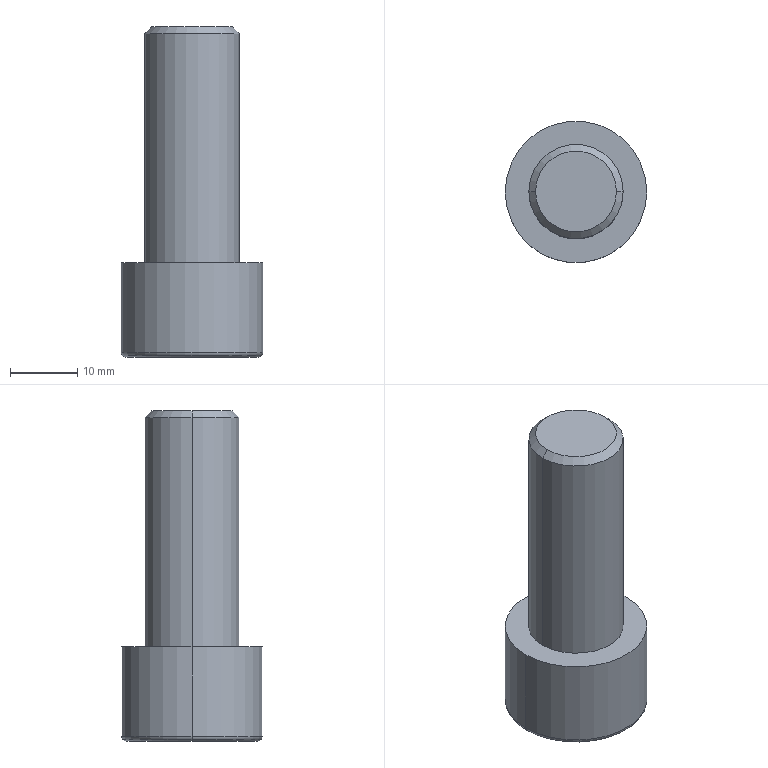Part | Creo | 1 solid | 20 faces | box 21 x 21 x 49 mm | volume 9057 mm3 | plane 10 | cylinder 4 | torus 4 | cone 2 | commonest cylinder face diameters 14 x2 21 x2
STEP:
#1=CARTESIAN_POINT('',(-272.,347.,-256.5));
#2=VERTEX_POINT('',#1);
#3=CARTESIAN_POINT('',(-258.,347.,-256.5));
#4=VERTEX_POINT('',#3);
#5=CARTESIAN_POINT('',(-265.,347.,-256.5));
#6=DIRECTION('',(0.,0.,1.));
#7=DIRECTION('',(-1.,0.,0.));
#8=AXIS2_PLACEMENT_3D('',#5,#6,#7);
#9=CIRCLE('',#8,7.);
#10=EDGE_CURVE('',#2,#4,#9,.T.);
#11=ORIENTED_EDGE('',*,*,#10,.T.);
#12=CARTESIAN_POINT('',(-258.,347.,-290.5));
#13=VERTEX_POINT('',#12);
#14=CARTESIAN_POINT('',(-258.,347.,-290.5));
#15=DIRECTION('',(0.,0.,1.));
#16=VECTOR('',#15,34.);
#17=LINE('',#14,#16);
#18=EDGE_CURVE('',#13,#4,#17,.T.);
#19=ORIENTED_EDGE('',*,*,#18,.F.);
#20=CARTESIAN_POINT('',(-272.,347.,-290.5));
#21=VERTEX_POINT('',#20);
#22=CARTESIAN_POINT('',(-265.,347.,-290.5));
#23=DIRECTION('',(0.,0.,-1.));
#24=DIRECTION('',(1.,0.,0.));
#25=AXIS2_PLACEMENT_3D('',#22,#23,#24);
#26=CIRCLE('',#25,7.);
#27=EDGE_CURVE('',#13,#21,#26,.T.);
#28=ORIENTED_EDGE('',*,*,#27,.T.);
#29=CARTESIAN_POINT('',(-272.,347.,-290.5));
#30=DIRECTION('',(0.,0.,1.));
#31=VECTOR('',#30,34.);
#32=LINE('',#29,#31);
#33=EDGE_CURVE('',#21,#2,#32,.T.);
#34=ORIENTED_EDGE('',*,*,#33,.T.);
#35=EDGE_LOOP('',(#11,#19,#28,#34));
#36=FACE_OUTER_BOUND('',#35,.F.);
#37=CARTESIAN_POINT('',(-265.,347.,-290.5));
#38=DIRECTION('',(0.,0.,1.));
#39=DIRECTION('',(-1.,0.,0.));
#40=AXIS2_PLACEMENT_3D('',#37,#38,#39);
#41=CYLINDRICAL_SURFACE('',#40,7.);
#42=ADVANCED_FACE('',(#36),#41,.T.);
#43=CARTESIAN_POINT('',(-271.,347.,-255.5));
#44=VERTEX_POINT('',#43);
#45=CARTESIAN_POINT('',(-259.,347.,-255.5));
#46=VERTEX_POINT('',#45);
#47=CARTESIAN_POINT('',(-265.,347.,-255.5));
#48=DIRECTION('',(0.,0.,1.));
#49=DIRECTION('',(-1.,0.,0.));
#50=AXIS2_PLACEMENT_3D('',#47,#48,#49);
#51=CIRCLE('',#50,6.);
#52=EDGE_CURVE('',#44,#46,#51,.T.);
#53=ORIENTED_EDGE('',*,*,#52,.T.);
#54=CARTESIAN_POINT('',(-259.,347.,-255.5));
#55=DIRECTION('',(0.7071,0.,-0.7071));
#56=VECTOR('',#55,1.414);
#57=LINE('',#54,#56);
#58=EDGE_CURVE('',#46,#4,#57,.T.);
#59=ORIENTED_EDGE('',*,*,#58,.T.);
#60=ORIENTED_EDGE('',*,*,#10,.F.);
#61=CARTESIAN_POINT('',(-271.,347.,-255.5));
#62=DIRECTION('',(-0.7071,0.,-0.7071));
#63=VECTOR('',#62,1.414);
#64=LINE('',#61,#63);
#65=EDGE_CURVE('',#44,#2,#64,.T.);
#66=ORIENTED_EDGE('',*,*,#65,.F.);
#67=EDGE_LOOP('',(#53,#59,#60,#66));
#68=FACE_OUTER_BOUND('',#67,.F.);
#69=CARTESIAN_POINT('',(-265.,347.,-256.));
#70=DIRECTION('',(0.,0.,-1.));
#71=DIRECTION('',(1.,0.,0.));
#72=AXIS2_PLACEMENT_3D('',#69,#70,#71);
#73=CONICAL_SURFACE('',#72,6.5,45.);
#74=ADVANCED_FACE('',(#68),#73,.T.);
#75=CARTESIAN_POINT('',(-265.,347.,-255.5));
#76=DIRECTION('',(0.,0.,1.));
#77=DIRECTION('',(1.,0.,0.));
#78=AXIS2_PLACEMENT_3D('',#75,#76,#77);
#79=CIRCLE('',#78,6.);
#80=EDGE_CURVE('',#46,#44,#79,.T.);
#81=ORIENTED_EDGE('',*,*,#80,.F.);
#82=ORIENTED_EDGE('',*,*,#52,.F.);
#83=EDGE_LOOP('',(#81,#82));
#84=FACE_OUTER_BOUND('',#83,.F.);
#85=CARTESIAN_POINT('',(-265.,347.,-255.5));
#86=DIRECTION('',(0.,0.,-1.));
#87=DIRECTION('',(1.,0.,0.));
#88=AXIS2_PLACEMENT_3D('',#85,#86,#87);
#89=PLANE('',#88);
#90=ADVANCED_FACE('',(#84),#89,.F.);
#91=ORIENTED_EDGE('',*,*,#80,.T.);
#92=ORIENTED_EDGE('',*,*,#65,.T.);
#93=CARTESIAN_POINT('',(-265.,347.,-256.5));
#94=DIRECTION('',(0.,0.,1.));
#95=DIRECTION('',(1.,0.,0.));
#96=AXIS2_PLACEMENT_3D('',#93,#94,#95);
#97=CIRCLE('',#96,7.);
#98=EDGE_CURVE('',#4,#2,#97,.T.);
#99=ORIENTED_EDGE('',*,*,#98,.F.);
#100=ORIENTED_EDGE('',*,*,#58,.F.);
#101=EDGE_LOOP('',(#91,#92,#99,#100));
#102=FACE_OUTER_BOUND('',#101,.F.);
#103=CARTESIAN_POINT('',(-265.,347.,-256.));
#104=DIRECTION('',(0.,0.,-1.));
#105=DIRECTION('',(1.,0.,0.));
#106=AXIS2_PLACEMENT_3D('',#103,#104,#105);
#107=CONICAL_SURFACE('',#106,6.5,45.);
#108=ADVANCED_FACE('',(#102),#107,.T.);
#109=ORIENTED_EDGE('',*,*,#98,.T.);
#110=ORIENTED_EDGE('',*,*,#33,.F.);
#111=CARTESIAN_POINT('',(-265.,347.,-290.5));
#112=DIRECTION('',(0.,0.,-1.));
#113=DIRECTION('',(-1.,0.,0.));
#114=AXIS2_PLACEMENT_3D('',#111,#112,#113);
#115=CIRCLE('',#114,7.);
#116=EDGE_CURVE('',#21,#13,#115,.T.);
#117=ORIENTED_EDGE('',*,*,#116,.T.);
#118=ORIENTED_EDGE('',*,*,#18,.T.);
#119=EDGE_LOOP('',(#109,#110,#117,#118));
#120=FACE_OUTER_BOUND('',#119,.F.);
#121=CARTESIAN_POINT('',(-265.,347.,-290.5));
#122=DIRECTION('',(0.,0.,1.));
#123=DIRECTION('',(-1.,0.,0.));
#124=AXIS2_PLACEMENT_3D('',#121,#122,#123);
#125=CYLINDRICAL_SURFACE('',#124,7.);
#126=ADVANCED_FACE('',(#120),#125,.T.);
#127=CARTESIAN_POINT('',(-254.5,347.,-290.5));
#128=VERTEX_POINT('',#127);
#129=CARTESIAN_POINT('',(-275.5,347.,-290.5));
#130=VERTEX_POINT('',#129);
#131=CARTESIAN_POINT('',(-265.,347.,-290.5));
#132=DIRECTION('',(0.,0.,1.));
#133=DIRECTION('',(1.,0.,0.));
#134=AXIS2_PLACEMENT_3D('',#131,#132,#133);
#135=CIRCLE('',#134,10.5);
#136=EDGE_CURVE('',#128,#130,#135,.T.);
#137=ORIENTED_EDGE('',*,*,#136,.F.);
#138=CARTESIAN_POINT('',(-265.,347.,-290.5));
#139=DIRECTION('',(0.,0.,1.));
#140=DIRECTION('',(-1.,0.,0.));
#141=AXIS2_PLACEMENT_3D('',#138,#139,#140);
#142=CIRCLE('',#141,10.5);
#143=EDGE_CURVE('',#130,#128,#142,.T.);
#144=ORIENTED_EDGE('',*,*,#143,.F.);
#145=EDGE_LOOP('',(#137,#144));
#146=FACE_OUTER_BOUND('',#145,.F.);
#147=ORIENTED_EDGE('',*,*,#27,.F.);
#148=ORIENTED_EDGE('',*,*,#116,.F.);
#149=EDGE_LOOP('',(#147,#148));
#150=FACE_BOUND('',#149,.F.);
#151=CARTESIAN_POINT('',(-265.,347.,-290.5));
#152=DIRECTION('',(0.,0.,1.));
#153=DIRECTION('',(-1.,0.,0.));
#154=AXIS2_PLACEMENT_3D('',#151,#152,#153);
#155=PLANE('',#154);
#156=ADVANCED_FACE('',(#146,#150),#155,.T.);
#157=CARTESIAN_POINT('',(-275.5,347.,-303.8));
#158=VERTEX_POINT('',#157);
#159=CARTESIAN_POINT('',(-254.5,347.,-303.8));
#160=VERTEX_POINT('',#159);
#161=CARTESIAN_POINT('',(-265.,347.,-303.8));
#162=DIRECTION('',(0.,0.,-1.));
#163=DIRECTION('',(-1.,0.,0.));
#164=AXIS2_PLACEMENT_3D('',#161,#162,#163);
#165=CIRCLE('',#164,10.5);
#166=EDGE_CURVE('',#158,#160,#165,.T.);
#167=ORIENTED_EDGE('',*,*,#166,.T.);
#168=CARTESIAN_POINT('',(-254.5,347.,-290.5));
#169=DIRECTION('',(0.,0.,-1.));
#170=VECTOR('',#169,13.3);
#171=LINE('',#168,#170);
#172=EDGE_CURVE('',#128,#160,#171,.T.);
#173=ORIENTED_EDGE('',*,*,#172,.F.);
#174=ORIENTED_EDGE('',*,*,#136,.T.);
#175=CARTESIAN_POINT('',(-275.5,347.,-290.5));
#176=DIRECTION('',(0.,0.,-1.));
#177=VECTOR('',#176,13.3);
#178=LINE('',#175,#177);
#179=EDGE_CURVE('',#130,#158,#178,.T.);
#180=ORIENTED_EDGE('',*,*,#179,.T.);
#181=EDGE_LOOP('',(#167,#173,#174,#180));
#182=FACE_OUTER_BOUND('',#181,.F.);
#183=CARTESIAN_POINT('',(-265.,347.,-290.5));
#184=DIRECTION('',(0.,0.,-1.));
#185=DIRECTION('',(1.,0.,0.));
#186=AXIS2_PLACEMENT_3D('',#183,#184,#185);
#187=CYLINDRICAL_SURFACE('',#186,10.5);
#188=ADVANCED_FACE('',(#182),#187,.T.);
#189=ORIENTED_EDGE('',*,*,#166,.F.);
#190=CARTESIAN_POINT('',(-275.295,347.,-304.295));
#191=VERTEX_POINT('',#190);
#192=CARTESIAN_POINT('',(-274.8,347.,-303.8));
#193=DIRECTION('',(0.,-1.,0.));
#194=DIRECTION('',(-1.,0.,0.));
#195=AXIS2_PLACEMENT_3D('',#192,#193,#194);
#196=CIRCLE('',#195,0.7);
#197=EDGE_CURVE('',#158,#191,#196,.T.);
#198=ORIENTED_EDGE('',*,*,#197,.T.);
#199=CARTESIAN_POINT('',(-254.705,347.,-304.295));
#200=VERTEX_POINT('',#199);
#201=CARTESIAN_POINT('',(-265.,347.,-304.295));
#202=DIRECTION('',(0.,0.,-1.));
#203=DIRECTION('',(-1.,0.,0.));
#204=AXIS2_PLACEMENT_3D('',#201,#202,#203);
#205=CIRCLE('',#204,10.295);
#206=EDGE_CURVE('',#191,#200,#205,.T.);
#207=ORIENTED_EDGE('',*,*,#206,.T.);
#208=CARTESIAN_POINT('',(-255.2,347.,-303.8));
#209=DIRECTION('',(0.,1.,0.));
#210=DIRECTION('',(1.,0.,0.));
#211=AXIS2_PLACEMENT_3D('',#208,#209,#210);
#212=CIRCLE('',#211,0.7);
#213=EDGE_CURVE('',#160,#200,#212,.T.);
#214=ORIENTED_EDGE('',*,*,#213,.F.);
#215=EDGE_LOOP('',(#189,#198,#207,#214));
#216=FACE_OUTER_BOUND('',#215,.F.);
#217=CARTESIAN_POINT('',(-265.,347.,-303.8));
#218=DIRECTION('',(0.,0.,-1.));
#219=DIRECTION('',(1.,0.,0.));
#220=AXIS2_PLACEMENT_3D('',#217,#218,#219);
#221=TOROIDAL_SURFACE('',#220,9.8,0.7);
#222=ADVANCED_FACE('',(#216),#221,.T.);
#223=CARTESIAN_POINT('',(-265.,347.,-303.8));
#224=DIRECTION('',(0.,0.,-1.));
#225=DIRECTION('',(1.,0.,0.));
#226=AXIS2_PLACEMENT_3D('',#223,#224,#225);
#227=CIRCLE('',#226,10.5);
#228=EDGE_CURVE('',#160,#158,#227,.T.);
#229=ORIENTED_EDGE('',*,*,#228,.F.);
#230=ORIENTED_EDGE('',*,*,#213,.T.);
#231=CARTESIAN_POINT('',(-265.,347.,-304.295));
#232=DIRECTION('',(0.,0.,-1.));
#233=DIRECTION('',(1.,0.,0.));
#234=AXIS2_PLACEMENT_3D('',#231,#232,#233);
#235=CIRCLE('',#234,10.295);
#236=EDGE_CURVE('',#200,#191,#235,.T.);
#237=ORIENTED_EDGE('',*,*,#236,.T.);
#238=ORIENTED_EDGE('',*,*,#197,.F.);
#239=EDGE_LOOP('',(#229,#230,#237,#238));
#240=FACE_OUTER_BOUND('',#239,.F.);
#241=CARTESIAN_POINT('',(-265.,347.,-303.8));
#242=DIRECTION('',(0.,0.,-1.));
#243=DIRECTION('',(1.,0.,0.));
#244=AXIS2_PLACEMENT_3D('',#241,#242,#243);
#245=TOROIDAL_SURFACE('',#244,9.8,0.7);
#246=ADVANCED_FACE('',(#240),#245,.T.);
#247=ORIENTED_EDGE('',*,*,#228,.T.);
#248=ORIENTED_EDGE('',*,*,#179,.F.);
#249=ORIENTED_EDGE('',*,*,#143,.T.);
#250=ORIENTED_EDGE('',*,*,#172,.T.);
#251=EDGE_LOOP('',(#247,#248,#249,#250));
#252=FACE_OUTER_BOUND('',#251,.F.);
#253=CARTESIAN_POINT('',(-265.,347.,-290.5));
#254=DIRECTION('',(0.,0.,-1.));
#255=DIRECTION('',(1.,0.,0.));
#256=AXIS2_PLACEMENT_3D('',#253,#254,#255);
#257=CYLINDRICAL_SURFACE('',#256,10.5);
#258=ADVANCED_FACE('',(#252),#257,.T.);
#259=CARTESIAN_POINT('',(-255.2,347.,-304.5));
#260=VERTEX_POINT('',#259);
#261=CARTESIAN_POINT('',(-274.8,347.,-304.5));
#262=VERTEX_POINT('',#261);
#263=CARTESIAN_POINT('',(-265.,347.,-304.5));
#264=DIRECTION('',(0.,0.,-1.));
#265=DIRECTION('',(1.,0.,0.));
#266=AXIS2_PLACEMENT_3D('',#263,#264,#265);
#267=CIRCLE('',#266,9.8);
#268=EDGE_CURVE('',#260,#262,#267,.T.);
#269=ORIENTED_EDGE('',*,*,#268,.T.);
#270=CARTESIAN_POINT('',(-274.8,347.,-303.8));
#271=DIRECTION('',(0.,-1.,0.));
#272=DIRECTION('',(-0.7071,0.,-0.7071));
#273=AXIS2_PLACEMENT_3D('',#270,#271,#272);
#274=CIRCLE('',#273,0.7);
#275=EDGE_CURVE('',#191,#262,#274,.T.);
#276=ORIENTED_EDGE('',*,*,#275,.F.);
#277=ORIENTED_EDGE('',*,*,#236,.F.);
#278=CARTESIAN_POINT('',(-255.2,347.,-303.8));
#279=DIRECTION('',(0.,1.,0.));
#280=DIRECTION('',(0.7071,0.,-0.7071));
#281=AXIS2_PLACEMENT_3D('',#278,#279,#280);
#282=CIRCLE('',#281,0.7);
#283=EDGE_CURVE('',#200,#260,#282,.T.);
#284=ORIENTED_EDGE('',*,*,#283,.T.);
#285=EDGE_LOOP('',(#269,#276,#277,#284));
#286=FACE_OUTER_BOUND('',#285,.F.);
#287=CARTESIAN_POINT('',(-265.,347.,-303.8));
#288=DIRECTION('',(0.,0.,-1.));
#289=DIRECTION('',(1.,0.,0.));
#290=AXIS2_PLACEMENT_3D('',#287,#288,#289);
#291=TOROIDAL_SURFACE('',#290,9.8,0.7);
#292=ADVANCED_FACE('',(#286),#291,.T.);
#293=ORIENTED_EDGE('',*,*,#268,.F.);
#294=CARTESIAN_POINT('',(-265.,347.,-304.5));
#295=DIRECTION('',(0.,0.,-1.));
#296=DIRECTION('',(-1.,0.,0.));
#297=AXIS2_PLACEMENT_3D('',#294,#295,#296);
#298=CIRCLE('',#297,9.8);
#299=EDGE_CURVE('',#262,#260,#298,.T.);
#300=ORIENTED_EDGE('',*,*,#299,.F.);
#301=EDGE_LOOP('',(#293,#300));
#302=FACE_OUTER_BOUND('',#301,.F.);
#303=CARTESIAN_POINT('',(-261.536,353.,-304.5));
#304=VERTEX_POINT('',#303);
#305=CARTESIAN_POINT('',(-268.464,353.,-304.5));
#306=VERTEX_POINT('',#305);
#307=CARTESIAN_POINT('',(-261.536,353.,-304.5));
#308=DIRECTION('',(-1.,0.,0.));
#309=VECTOR('',#308,6.928);
#310=LINE('',#307,#309);
#311=EDGE_CURVE('',#304,#306,#310,.T.);
#312=ORIENTED_EDGE('',*,*,#311,.F.);
#313=CARTESIAN_POINT('',(-258.072,347.,-304.5));
#314=VERTEX_POINT('',#313);
#315=CARTESIAN_POINT('',(-258.072,347.,-304.5));
#316=DIRECTION('',(-0.5,0.866,0.));
#317=VECTOR('',#316,6.928);
#318=LINE('',#315,#317);
#319=EDGE_CURVE('',#314,#304,#318,.T.);
#320=ORIENTED_EDGE('',*,*,#319,.F.);
#321=CARTESIAN_POINT('',(-261.536,341.,-304.5));
#322=VERTEX_POINT('',#321);
#323=CARTESIAN_POINT('',(-261.536,341.,-304.5));
#324=DIRECTION('',(0.5,0.866,0.));
#325=VECTOR('',#324,6.928);
#326=LINE('',#323,#325);
#327=EDGE_CURVE('',#322,#314,#326,.T.);
#328=ORIENTED_EDGE('',*,*,#327,.F.);
#329=CARTESIAN_POINT('',(-268.464,341.,-304.5));
#330=VERTEX_POINT('',#329);
#331=CARTESIAN_POINT('',(-268.464,341.,-304.5));
#332=DIRECTION('',(1.,0.,0.));
#333=VECTOR('',#332,6.928);
#334=LINE('',#331,#333);
#335=EDGE_CURVE('',#330,#322,#334,.T.);
#336=ORIENTED_EDGE('',*,*,#335,.F.);
#337=CARTESIAN_POINT('',(-271.928,347.,-304.5));
#338=VERTEX_POINT('',#337);
#339=CARTESIAN_POINT('',(-271.928,347.,-304.5));
#340=DIRECTION('',(0.5,-0.866,0.));
#341=VECTOR('',#340,6.928);
#342=LINE('',#339,#341);
#343=EDGE_CURVE('',#338,#330,#342,.T.);
#344=ORIENTED_EDGE('',*,*,#343,.F.);
#345=CARTESIAN_POINT('',(-268.464,353.,-304.5));
#346=DIRECTION('',(-0.5,-0.866,0.));
#347=VECTOR('',#346,6.928);
#348=LINE('',#345,#347);
#349=EDGE_CURVE('',#306,#338,#348,.T.);
#350=ORIENTED_EDGE('',*,*,#349,.F.);
#351=EDGE_LOOP('',(#312,#320,#328,#336,#344,#350));
#352=FACE_BOUND('',#351,.F.);
#353=CARTESIAN_POINT('',(-265.,347.,-304.5));
#354=DIRECTION('',(0.,0.,-1.));
#355=DIRECTION('',(1.,0.,0.));
#356=AXIS2_PLACEMENT_3D('',#353,#354,#355);
#357=PLANE('',#356);
#358=ADVANCED_FACE('',(#302,#352),#357,.T.);
#359=ORIENTED_EDGE('',*,*,#299,.T.);
#360=ORIENTED_EDGE('',*,*,#283,.F.);
#361=ORIENTED_EDGE('',*,*,#206,.F.);
#362=ORIENTED_EDGE('',*,*,#275,.T.);
#363=EDGE_LOOP('',(#359,#360,#361,#362));
#364=FACE_OUTER_BOUND('',#363,.F.);
#365=CARTESIAN_POINT('',(-265.,347.,-303.8));
#366=DIRECTION('',(0.,0.,-1.));
#367=DIRECTION('',(1.,0.,0.));
#368=AXIS2_PLACEMENT_3D('',#365,#366,#367);
#369=TOROIDAL_SURFACE('',#368,9.8,0.7);
#370=ADVANCED_FACE('',(#364),#369,.T.);
#371=ORIENTED_EDGE('',*,*,#311,.T.);
#372=CARTESIAN_POINT('',(-268.464,353.,-295.26));
#373=VERTEX_POINT('',#372);
#374=CARTESIAN_POINT('',(-268.464,353.,-304.5));
#375=DIRECTION('',(0.,0.,1.));
#376=VECTOR('',#375,9.24);
#377=LINE('',#374,#376);
#378=EDGE_CURVE('',#306,#373,#377,.T.);
#379=ORIENTED_EDGE('',*,*,#378,.T.);
#380=CARTESIAN_POINT('',(-261.536,353.,-295.26));
#381=VERTEX_POINT('',#380);
#382=CARTESIAN_POINT('',(-261.536,353.,-295.26));
#383=DIRECTION('',(-1.,0.,0.));
#384=VECTOR('',#383,6.928);
#385=LINE('',#382,#384);
#386=EDGE_CURVE('',#381,#373,#385,.T.);
#387=ORIENTED_EDGE('',*,*,#386,.F.);
#388=CARTESIAN_POINT('',(-261.536,353.,-304.5));
#389=DIRECTION('',(0.,0.,1.));
#390=VECTOR('',#389,9.24);
#391=LINE('',#388,#390);
#392=EDGE_CURVE('',#304,#381,#391,.T.);
#393=ORIENTED_EDGE('',*,*,#392,.F.);
#394=EDGE_LOOP('',(#371,#379,#387,#393));
#395=FACE_OUTER_BOUND('',#394,.F.);
#396=CARTESIAN_POINT('',(-268.464,353.,-295.26));
#397=DIRECTION('',(0.,1.,0.));
#398=DIRECTION('',(0.,0.,1.));
#399=AXIS2_PLACEMENT_3D('',#396,#397,#398);
#400=PLANE('',#399);
#401=ADVANCED_FACE('',(#395),#400,.F.);
#402=ORIENTED_EDGE('',*,*,#349,.T.);
#403=CARTESIAN_POINT('',(-271.928,347.,-295.26));
#404=VERTEX_POINT('',#403);
#405=CARTESIAN_POINT('',(-271.928,347.,-304.5));
#406=DIRECTION('',(0.,0.,1.));
#407=VECTOR('',#406,9.24);
#408=LINE('',#405,#407);
#409=EDGE_CURVE('',#338,#404,#408,.T.);
#410=ORIENTED_EDGE('',*,*,#409,.T.);
#411=CARTESIAN_POINT('',(-271.928,347.,-295.26));
#412=DIRECTION('',(0.5,0.866,0.));
#413=VECTOR('',#412,6.928);
#414=LINE('',#411,#413);
#415=EDGE_CURVE('',#404,#373,#414,.T.);
#416=ORIENTED_EDGE('',*,*,#415,.T.);
#417=ORIENTED_EDGE('',*,*,#378,.F.);
#418=EDGE_LOOP('',(#402,#410,#416,#417));
#419=FACE_OUTER_BOUND('',#418,.F.);
#420=CARTESIAN_POINT('',(-271.928,347.,-295.26));
#421=DIRECTION('',(-0.866,0.5,0.));
#422=DIRECTION('',(0.5,0.866,0.));
#423=AXIS2_PLACEMENT_3D('',#420,#421,#422);
#424=PLANE('',#423);
#425=ADVANCED_FACE('',(#419),#424,.F.);
#426=ORIENTED_EDGE('',*,*,#343,.T.);
#427=CARTESIAN_POINT('',(-268.464,341.,-295.26));
#428=VERTEX_POINT('',#427);
#429=CARTESIAN_POINT('',(-268.464,341.,-304.5));
#430=DIRECTION('',(0.,0.,1.));
#431=VECTOR('',#430,9.24);
#432=LINE('',#429,#431);
#433=EDGE_CURVE('',#330,#428,#432,.T.);
#434=ORIENTED_EDGE('',*,*,#433,.T.);
#435=CARTESIAN_POINT('',(-268.464,341.,-295.26));
#436=DIRECTION('',(-0.5,0.866,0.));
#437=VECTOR('',#436,6.928);
#438=LINE('',#435,#437);
#439=EDGE_CURVE('',#428,#404,#438,.T.);
#440=ORIENTED_EDGE('',*,*,#439,.T.);
#441=ORIENTED_EDGE('',*,*,#409,.F.);
#442=EDGE_LOOP('',(#426,#434,#440,#441));
#443=FACE_OUTER_BOUND('',#442,.F.);
#444=CARTESIAN_POINT('',(-268.464,341.,-295.26));
#445=DIRECTION('',(-0.866,-0.5,0.));
#446=DIRECTION('',(-0.5,0.866,0.));
#447=AXIS2_PLACEMENT_3D('',#444,#445,#446);
#448=PLANE('',#447);
#449=ADVANCED_FACE('',(#443),#448,.F.);
#450=ORIENTED_EDGE('',*,*,#335,.T.);
#451=CARTESIAN_POINT('',(-261.536,341.,-295.26));
#452=VERTEX_POINT('',#451);
#453=CARTESIAN_POINT('',(-261.536,341.,-304.5));
#454=DIRECTION('',(0.,0.,1.));
#455=VECTOR('',#454,9.24);
#456=LINE('',#453,#455);
#457=EDGE_CURVE('',#322,#452,#456,.T.);
#458=ORIENTED_EDGE('',*,*,#457,.T.);
#459=CARTESIAN_POINT('',(-268.464,341.,-295.26));
#460=DIRECTION('',(1.,0.,0.));
#461=VECTOR('',#460,6.928);
#462=LINE('',#459,#461);
#463=EDGE_CURVE('',#428,#452,#462,.T.);
#464=ORIENTED_EDGE('',*,*,#463,.F.);
#465=ORIENTED_EDGE('',*,*,#433,.F.);
#466=EDGE_LOOP('',(#450,#458,#464,#465));
#467=FACE_OUTER_BOUND('',#466,.F.);
#468=CARTESIAN_POINT('',(-261.536,341.,-295.26));
#469=DIRECTION('',(0.,-1.,0.));
#470=DIRECTION('',(0.,0.,-1.));
#471=AXIS2_PLACEMENT_3D('',#468,#469,#470);
#472=PLANE('',#471);
#473=ADVANCED_FACE('',(#467),#472,.F.);
#474=ORIENTED_EDGE('',*,*,#327,.T.);
#475=CARTESIAN_POINT('',(-258.072,347.,-295.26));
#476=VERTEX_POINT('',#475);
#477=CARTESIAN_POINT('',(-258.072,347.,-304.5));
#478=DIRECTION('',(0.,0.,1.));
#479=VECTOR('',#478,9.24);
#480=LINE('',#477,#479);
#481=EDGE_CURVE('',#314,#476,#480,.T.);
#482=ORIENTED_EDGE('',*,*,#481,.T.);
#483=CARTESIAN_POINT('',(-258.072,347.,-295.26));
#484=DIRECTION('',(-0.5,-0.866,0.));
#485=VECTOR('',#484,6.928);
#486=LINE('',#483,#485);
#487=EDGE_CURVE('',#476,#452,#486,.T.);
#488=ORIENTED_EDGE('',*,*,#487,.T.);
#489=ORIENTED_EDGE('',*,*,#457,.F.);
#490=EDGE_LOOP('',(#474,#482,#488,#489));
#491=FACE_OUTER_BOUND('',#490,.F.);
#492=CARTESIAN_POINT('',(-258.072,347.,-295.26));
#493=DIRECTION('',(0.866,-0.5,0.));
#494=DIRECTION('',(-0.5,-0.866,0.));
#495=AXIS2_PLACEMENT_3D('',#492,#493,#494);
#496=PLANE('',#495);
#497=ADVANCED_FACE('',(#491),#496,.F.);
#498=ORIENTED_EDGE('',*,*,#319,.T.);
#499=ORIENTED_EDGE('',*,*,#392,.T.);
#500=CARTESIAN_POINT('',(-261.536,353.,-295.26));
#501=DIRECTION('',(0.5,-0.866,0.));
#502=VECTOR('',#501,6.928);
#503=LINE('',#500,#502);
#504=EDGE_CURVE('',#381,#476,#503,.T.);
#505=ORIENTED_EDGE('',*,*,#504,.T.);
#506=ORIENTED_EDGE('',*,*,#481,.F.);
#507=EDGE_LOOP('',(#498,#499,#505,#506));
#508=FACE_OUTER_BOUND('',#507,.F.);
#509=CARTESIAN_POINT('',(-261.536,353.,-295.26));
#510=DIRECTION('',(0.866,0.5,0.));
#511=DIRECTION('',(0.5,-0.866,0.));
#512=AXIS2_PLACEMENT_3D('',#509,#510,#511);
#513=PLANE('',#512);
#514=ADVANCED_FACE('',(#508),#513,.F.);
#515=ORIENTED_EDGE('',*,*,#386,.T.);
#516=ORIENTED_EDGE('',*,*,#415,.F.);
#517=ORIENTED_EDGE('',*,*,#439,.F.);
#518=ORIENTED_EDGE('',*,*,#463,.T.);
#519=ORIENTED_EDGE('',*,*,#487,.F.);
#520=ORIENTED_EDGE('',*,*,#504,.F.);
#521=EDGE_LOOP('',(#515,#516,#517,#518,#519,#520));
#522=FACE_OUTER_BOUND('',#521,.F.);
#523=CARTESIAN_POINT('',(-261.536,353.,-295.26));
#524=DIRECTION('',(0.,0.,-1.));
#525=DIRECTION('',(1.,0.,0.));
#526=AXIS2_PLACEMENT_3D('',#523,#524,#525);
#527=PLANE('',#526);
#528=ADVANCED_FACE('',(#522),#527,.T.);
#529=CLOSED_SHELL('',(#42,#74,#90,#108,#126,#156,#188,#222,#246,#258,#292,#358,#370,#401,#425,#449,#473,#497,#514,#528));
#530=MANIFOLD_SOLID_BREP('',#529);
#531=(LENGTH_UNIT()NAMED_UNIT(*)SI_UNIT(.MILLI.,.METRE.));
#532=UNCERTAINTY_MEASURE_WITH_UNIT(LENGTH_MEASURE(0.00573),#531,'','');
#533=(NAMED_UNIT(*)PLANE_ANGLE_UNIT()SI_UNIT($,.RADIAN.));
#534=PLANE_ANGLE_MEASURE_WITH_UNIT(PLANE_ANGLE_MEASURE(0.01745),#533);
#535=(CONVERSION_BASED_UNIT('DEGREE',#534)NAMED_UNIT(*)PLANE_ANGLE_UNIT());
#536=(NAMED_UNIT(*)SI_UNIT($,.STERADIAN.)SOLID_ANGLE_UNIT());
#537=(GEOMETRIC_REPRESENTATION_CONTEXT(3)GLOBAL_UNCERTAINTY_ASSIGNED_CONTEXT((#532))GLOBAL_UNIT_ASSIGNED_CONTEXT((#531,#535,#536))REPRESENTATION_CONTEXT('',''));
#538=ADVANCED_BREP_SHAPE_REPRESENTATION('',(#530),#537);